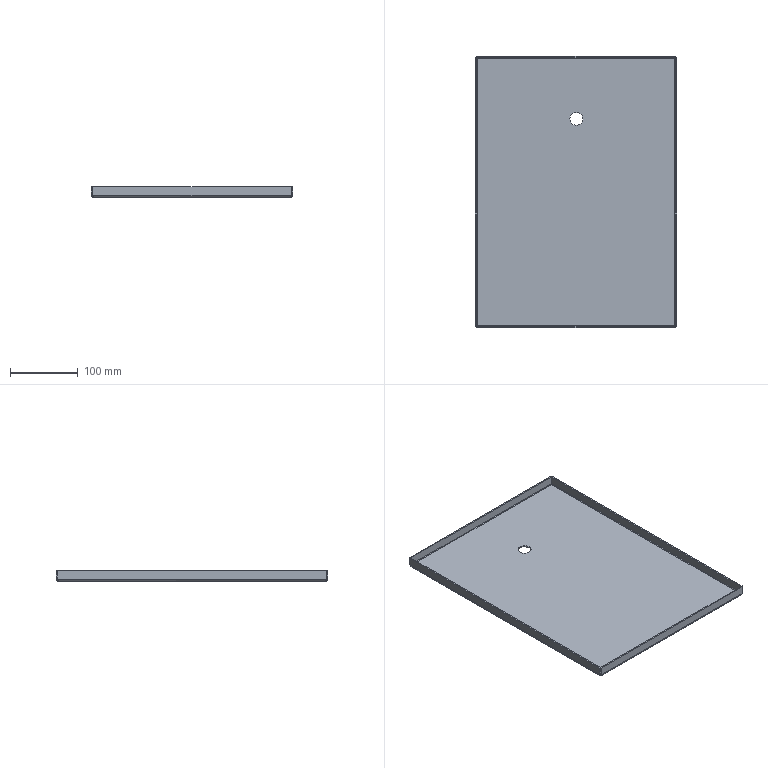Part | SolidWorks | features EdgeFlange 1, FlatPattern 1, ICE 1, SMBaseFlange 1, SheetMetal 1 | 1 solid | 40 faces | box 297 x 400 x 15 mm | volume 270369 mm3 | plane 22 | cylinder 10 | spline 8 | commonest cylinder face diameters 2 x4 6 x4 19 x2